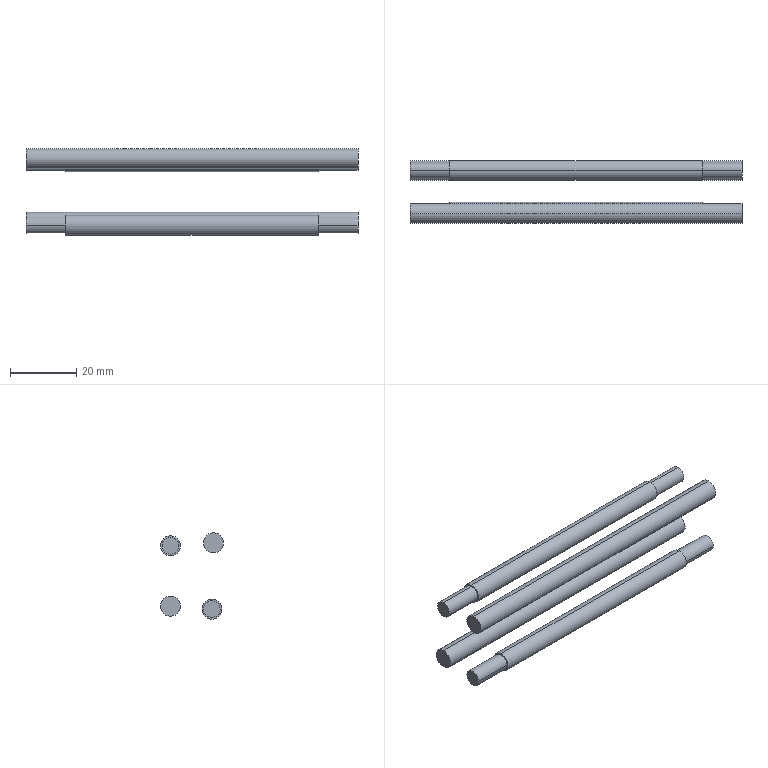Part | SolidWorks | features BaseBody 1, ICE 1 | 4 solids | 28 faces | box 100 x 19 x 26 mm | volume 10895 mm3 | cylinder 16 | plane 12 | commonest cylinder face diameters 5 x8 6 x8
STEP:
#1=CARTESIAN_POINT('',(-38.,-5.,-7.));
#2=VERTEX_POINT('',#1);
#3=CARTESIAN_POINT('',(-38.,-5.,-13.));
#4=VERTEX_POINT('',#3);
#5=CARTESIAN_POINT('',(-38.,-5.,-10.));
#6=DIRECTION('',(1.,0.,0.));
#7=DIRECTION('',(0.,0.,-1.));
#8=AXIS2_PLACEMENT_3D('',#5,#6,#7);
#9=CIRCLE('',#8,3.);
#10=EDGE_CURVE('',#2,#4,#9,.T.);
#11=ORIENTED_EDGE('',*,*,#10,.T.);
#12=CARTESIAN_POINT('',(38.,-5.,-13.));
#13=VERTEX_POINT('',#12);
#14=CARTESIAN_POINT('',(38.,-5.,-13.));
#15=DIRECTION('',(1.,0.,0.));
#16=VECTOR('',#15,1000.);
#17=LINE('',#14,#16);
#18=EDGE_CURVE('',#4,#13,#17,.T.);
#19=ORIENTED_EDGE('',*,*,#18,.T.);
#20=CARTESIAN_POINT('',(38.,-5.,-7.));
#21=VERTEX_POINT('',#20);
#22=CARTESIAN_POINT('',(38.,-5.,-10.));
#23=DIRECTION('',(-1.,0.,0.));
#24=DIRECTION('',(0.,0.,-1.));
#25=AXIS2_PLACEMENT_3D('',#22,#23,#24);
#26=CIRCLE('',#25,3.);
#27=EDGE_CURVE('',#13,#21,#26,.T.);
#28=ORIENTED_EDGE('',*,*,#27,.T.);
#29=CARTESIAN_POINT('',(38.,-5.,-7.));
#30=DIRECTION('',(1.,0.,0.));
#31=VECTOR('',#30,1000.);
#32=LINE('',#29,#31);
#33=EDGE_CURVE('',#2,#21,#32,.T.);
#34=ORIENTED_EDGE('',*,*,#33,.F.);
#35=EDGE_LOOP('',(#11,#19,#28,#34));
#36=FACE_OUTER_BOUND('',#35,.T.);
#37=CARTESIAN_POINT('',(38.,-5.,-10.));
#38=DIRECTION('',(1.,0.,0.));
#39=DIRECTION('',(0.,0.,1.));
#40=AXIS2_PLACEMENT_3D('',#37,#38,#39);
#41=CYLINDRICAL_SURFACE('',#40,3.);
#42=ADVANCED_FACE('',(#36),#41,.T.);
#43=CARTESIAN_POINT('',(-50.,-2.5,-10.));
#44=VERTEX_POINT('',#43);
#45=CARTESIAN_POINT('',(-50.,-7.5,-10.));
#46=VERTEX_POINT('',#45);
#47=CARTESIAN_POINT('',(-50.,-5.,-10.));
#48=DIRECTION('',(-1.,0.,0.));
#49=DIRECTION('',(0.,-1.,0.));
#50=AXIS2_PLACEMENT_3D('',#47,#48,#49);
#51=CIRCLE('',#50,2.5);
#52=EDGE_CURVE('',#44,#46,#51,.T.);
#53=ORIENTED_EDGE('',*,*,#52,.F.);
#54=CARTESIAN_POINT('',(-38.,-2.5,-10.));
#55=VERTEX_POINT('',#54);
#56=CARTESIAN_POINT('',(-50.,-2.5,-10.));
#57=DIRECTION('',(1.,0.,0.));
#58=VECTOR('',#57,1000.);
#59=LINE('',#56,#58);
#60=EDGE_CURVE('',#44,#55,#59,.T.);
#61=ORIENTED_EDGE('',*,*,#60,.T.);
#62=CARTESIAN_POINT('',(-38.,-7.5,-10.));
#63=VERTEX_POINT('',#62);
#64=CARTESIAN_POINT('',(-38.,-5.,-10.));
#65=DIRECTION('',(-1.,0.,0.));
#66=DIRECTION('',(0.,0.,-1.));
#67=AXIS2_PLACEMENT_3D('',#64,#65,#66);
#68=CIRCLE('',#67,2.5);
#69=EDGE_CURVE('',#55,#63,#68,.T.);
#70=ORIENTED_EDGE('',*,*,#69,.T.);
#71=CARTESIAN_POINT('',(-50.,-7.5,-10.));
#72=DIRECTION('',(1.,0.,0.));
#73=VECTOR('',#72,1000.);
#74=LINE('',#71,#73);
#75=EDGE_CURVE('',#46,#63,#74,.T.);
#76=ORIENTED_EDGE('',*,*,#75,.F.);
#77=EDGE_LOOP('',(#53,#61,#70,#76));
#78=FACE_OUTER_BOUND('',#77,.T.);
#79=CARTESIAN_POINT('',(-50.,-5.,-10.));
#80=DIRECTION('',(1.,0.,0.));
#81=DIRECTION('',(0.,-1.,0.));
#82=AXIS2_PLACEMENT_3D('',#79,#80,#81);
#83=CYLINDRICAL_SURFACE('',#82,2.5);
#84=ADVANCED_FACE('',(#78),#83,.T.);
#85=CARTESIAN_POINT('',(38.,-7.5,-10.));
#86=VERTEX_POINT('',#85);
#87=CARTESIAN_POINT('',(38.,-2.5,-10.));
#88=VERTEX_POINT('',#87);
#89=CARTESIAN_POINT('',(38.,-5.,-10.));
#90=DIRECTION('',(1.,0.,0.));
#91=DIRECTION('',(0.,0.,-1.));
#92=AXIS2_PLACEMENT_3D('',#89,#90,#91);
#93=CIRCLE('',#92,2.5);
#94=EDGE_CURVE('',#86,#88,#93,.T.);
#95=ORIENTED_EDGE('',*,*,#94,.T.);
#96=CARTESIAN_POINT('',(50.,-2.5,-10.));
#97=VERTEX_POINT('',#96);
#98=CARTESIAN_POINT('',(38.,-2.5,-10.));
#99=DIRECTION('',(1.,0.,0.));
#100=VECTOR('',#99,1000.);
#101=LINE('',#98,#100);
#102=EDGE_CURVE('',#88,#97,#101,.T.);
#103=ORIENTED_EDGE('',*,*,#102,.T.);
#104=CARTESIAN_POINT('',(50.,-7.5,-10.));
#105=VERTEX_POINT('',#104);
#106=CARTESIAN_POINT('',(50.,-5.,-10.));
#107=DIRECTION('',(-1.,0.,0.));
#108=DIRECTION('',(0.,-1.,0.));
#109=AXIS2_PLACEMENT_3D('',#106,#107,#108);
#110=CIRCLE('',#109,2.5);
#111=EDGE_CURVE('',#97,#105,#110,.T.);
#112=ORIENTED_EDGE('',*,*,#111,.T.);
#113=CARTESIAN_POINT('',(38.,-7.5,-10.));
#114=DIRECTION('',(1.,0.,0.));
#115=VECTOR('',#114,1000.);
#116=LINE('',#113,#115);
#117=EDGE_CURVE('',#86,#105,#116,.T.);
#118=ORIENTED_EDGE('',*,*,#117,.F.);
#119=EDGE_LOOP('',(#95,#103,#112,#118));
#120=FACE_OUTER_BOUND('',#119,.T.);
#121=CARTESIAN_POINT('',(38.,-5.,-10.));
#122=DIRECTION('',(1.,0.,0.));
#123=DIRECTION('',(0.,-1.,0.));
#124=AXIS2_PLACEMENT_3D('',#121,#122,#123);
#125=CYLINDRICAL_SURFACE('',#124,2.5);
#126=ADVANCED_FACE('',(#120),#125,.T.);
#127=CARTESIAN_POINT('',(50.,-5.,-10.));
#128=DIRECTION('',(-1.,0.,0.));
#129=DIRECTION('',(0.,-1.,0.));
#130=AXIS2_PLACEMENT_3D('',#127,#128,#129);
#131=CIRCLE('',#130,2.5);
#132=EDGE_CURVE('',#105,#97,#131,.T.);
#133=ORIENTED_EDGE('',*,*,#132,.F.);
#134=ORIENTED_EDGE('',*,*,#111,.F.);
#135=EDGE_LOOP('',(#133,#134));
#136=FACE_OUTER_BOUND('',#135,.T.);
#137=CARTESIAN_POINT('',(50.,-5.,-10.));
#138=DIRECTION('',(-1.,0.,0.));
#139=DIRECTION('',(0.,0.,1.));
#140=AXIS2_PLACEMENT_3D('',#137,#138,#139);
#141=PLANE('',#140);
#142=ADVANCED_FACE('',(#136),#141,.F.);
#143=ORIENTED_EDGE('',*,*,#102,.F.);
#144=CARTESIAN_POINT('',(38.,-5.,-10.));
#145=DIRECTION('',(1.,0.,0.));
#146=DIRECTION('',(0.,0.,-1.));
#147=AXIS2_PLACEMENT_3D('',#144,#145,#146);
#148=CIRCLE('',#147,2.5);
#149=EDGE_CURVE('',#88,#86,#148,.T.);
#150=ORIENTED_EDGE('',*,*,#149,.T.);
#151=ORIENTED_EDGE('',*,*,#117,.T.);
#152=ORIENTED_EDGE('',*,*,#132,.T.);
#153=EDGE_LOOP('',(#143,#150,#151,#152));
#154=FACE_OUTER_BOUND('',#153,.T.);
#155=CARTESIAN_POINT('',(38.,-5.,-10.));
#156=DIRECTION('',(1.,0.,0.));
#157=DIRECTION('',(0.,-1.,0.));
#158=AXIS2_PLACEMENT_3D('',#155,#156,#157);
#159=CYLINDRICAL_SURFACE('',#158,2.5);
#160=ADVANCED_FACE('',(#154),#159,.T.);
#161=CARTESIAN_POINT('',(38.,-5.,-10.));
#162=DIRECTION('',(-1.,0.,0.));
#163=DIRECTION('',(0.,0.,-1.));
#164=AXIS2_PLACEMENT_3D('',#161,#162,#163);
#165=CIRCLE('',#164,3.);
#166=EDGE_CURVE('',#21,#13,#165,.T.);
#167=ORIENTED_EDGE('',*,*,#166,.F.);
#168=ORIENTED_EDGE('',*,*,#27,.F.);
#169=EDGE_LOOP('',(#167,#168));
#170=FACE_OUTER_BOUND('',#169,.T.);
#171=ORIENTED_EDGE('',*,*,#94,.F.);
#172=ORIENTED_EDGE('',*,*,#149,.F.);
#173=EDGE_LOOP('',(#171,#172));
#174=FACE_BOUND('',#173,.T.);
#175=CARTESIAN_POINT('',(38.,0.,0.));
#176=DIRECTION('',(1.,0.,0.));
#177=DIRECTION('',(0.,0.,-1.));
#178=AXIS2_PLACEMENT_3D('',#175,#176,#177);
#179=PLANE('',#178);
#180=ADVANCED_FACE('',(#170,#174),#179,.T.);
#181=CARTESIAN_POINT('',(-50.,-5.,-10.));
#182=DIRECTION('',(-1.,0.,0.));
#183=DIRECTION('',(0.,-1.,0.));
#184=AXIS2_PLACEMENT_3D('',#181,#182,#183);
#185=CIRCLE('',#184,2.5);
#186=EDGE_CURVE('',#46,#44,#185,.T.);
#187=ORIENTED_EDGE('',*,*,#186,.T.);
#188=ORIENTED_EDGE('',*,*,#52,.T.);
#189=EDGE_LOOP('',(#187,#188));
#190=FACE_OUTER_BOUND('',#189,.T.);
#191=CARTESIAN_POINT('',(-50.,-7.5,-10.));
#192=DIRECTION('',(1.,0.,0.));
#193=DIRECTION('',(0.,1.,0.));
#194=AXIS2_PLACEMENT_3D('',#191,#192,#193);
#195=PLANE('',#194);
#196=ADVANCED_FACE('',(#190),#195,.F.);
#197=ORIENTED_EDGE('',*,*,#60,.F.);
#198=ORIENTED_EDGE('',*,*,#186,.F.);
#199=ORIENTED_EDGE('',*,*,#75,.T.);
#200=CARTESIAN_POINT('',(-38.,-5.,-10.));
#201=DIRECTION('',(-1.,0.,0.));
#202=DIRECTION('',(0.,0.,-1.));
#203=AXIS2_PLACEMENT_3D('',#200,#201,#202);
#204=CIRCLE('',#203,2.5);
#205=EDGE_CURVE('',#63,#55,#204,.T.);
#206=ORIENTED_EDGE('',*,*,#205,.T.);
#207=EDGE_LOOP('',(#197,#198,#199,#206));
#208=FACE_OUTER_BOUND('',#207,.T.);
#209=CARTESIAN_POINT('',(-50.,-5.,-10.));
#210=DIRECTION('',(1.,0.,0.));
#211=DIRECTION('',(0.,-1.,0.));
#212=AXIS2_PLACEMENT_3D('',#209,#210,#211);
#213=CYLINDRICAL_SURFACE('',#212,2.5);
#214=ADVANCED_FACE('',(#208),#213,.T.);
#215=ORIENTED_EDGE('',*,*,#10,.F.);
#216=CARTESIAN_POINT('',(-38.,-5.,-10.));
#217=DIRECTION('',(1.,0.,0.));
#218=DIRECTION('',(0.,0.,-1.));
#219=AXIS2_PLACEMENT_3D('',#216,#217,#218);
#220=CIRCLE('',#219,3.);
#221=EDGE_CURVE('',#4,#2,#220,.T.);
#222=ORIENTED_EDGE('',*,*,#221,.F.);
#223=EDGE_LOOP('',(#215,#222));
#224=FACE_OUTER_BOUND('',#223,.T.);
#225=ORIENTED_EDGE('',*,*,#205,.F.);
#226=ORIENTED_EDGE('',*,*,#69,.F.);
#227=EDGE_LOOP('',(#225,#226));
#228=FACE_BOUND('',#227,.T.);
#229=CARTESIAN_POINT('',(-38.,-5.,-10.));
#230=DIRECTION('',(1.,0.,0.));
#231=DIRECTION('',(0.,1.,0.));
#232=AXIS2_PLACEMENT_3D('',#229,#230,#231);
#233=PLANE('',#232);
#234=ADVANCED_FACE('',(#224,#228),#233,.F.);
#235=ORIENTED_EDGE('',*,*,#18,.F.);
#236=ORIENTED_EDGE('',*,*,#221,.T.);
#237=ORIENTED_EDGE('',*,*,#33,.T.);
#238=ORIENTED_EDGE('',*,*,#166,.T.);
#239=EDGE_LOOP('',(#235,#236,#237,#238));
#240=FACE_OUTER_BOUND('',#239,.T.);
#241=CARTESIAN_POINT('',(38.,-5.,-10.));
#242=DIRECTION('',(1.,0.,0.));
#243=DIRECTION('',(0.,0.,1.));
#244=AXIS2_PLACEMENT_3D('',#241,#242,#243);
#245=CYLINDRICAL_SURFACE('',#244,3.);
#246=ADVANCED_FACE('',(#240),#245,.T.);
#247=CLOSED_SHELL('',(#42,#84,#126,#142,#160,#180,#196,#214,#234,#246));
#248=MANIFOLD_SOLID_BREP('',#247);
#249=CARTESIAN_POINT('',(-50.,-5.5,13.));
#250=VERTEX_POINT('',#249);
#251=CARTESIAN_POINT('',(-50.,-5.5,7.));
#252=VERTEX_POINT('',#251);
#253=CARTESIAN_POINT('',(-50.,-5.5,10.));
#254=DIRECTION('',(1.,0.,0.));
#255=DIRECTION('',(0.,0.,-1.));
#256=AXIS2_PLACEMENT_3D('',#253,#254,#255);
#257=CIRCLE('',#256,3.);
#258=EDGE_CURVE('',#250,#252,#257,.T.);
#259=ORIENTED_EDGE('',*,*,#258,.T.);
#260=CARTESIAN_POINT('',(50.,-5.5,7.));
#261=VERTEX_POINT('',#260);
#262=CARTESIAN_POINT('',(50.,-5.5,7.));
#263=DIRECTION('',(1.,0.,0.));
#264=VECTOR('',#263,1000.);
#265=LINE('',#262,#264);
#266=EDGE_CURVE('',#252,#261,#265,.T.);
#267=ORIENTED_EDGE('',*,*,#266,.T.);
#268=CARTESIAN_POINT('',(50.,-5.5,13.));
#269=VERTEX_POINT('',#268);
#270=CARTESIAN_POINT('',(50.,-5.5,10.));
#271=DIRECTION('',(1.,0.,0.));
#272=DIRECTION('',(0.,0.,-1.));
#273=AXIS2_PLACEMENT_3D('',#270,#271,#272);
#274=CIRCLE('',#273,3.);
#275=EDGE_CURVE('',#269,#261,#274,.T.);
#276=ORIENTED_EDGE('',*,*,#275,.F.);
#277=CARTESIAN_POINT('',(50.,-5.5,13.));
#278=DIRECTION('',(1.,0.,0.));
#279=VECTOR('',#278,1000.);
#280=LINE('',#277,#279);
#281=EDGE_CURVE('',#250,#269,#280,.T.);
#282=ORIENTED_EDGE('',*,*,#281,.F.);
#283=EDGE_LOOP('',(#259,#267,#276,#282));
#284=FACE_OUTER_BOUND('',#283,.T.);
#285=CARTESIAN_POINT('',(50.,-5.5,10.));
#286=DIRECTION('',(1.,0.,0.));
#287=DIRECTION('',(0.,0.,1.));
#288=AXIS2_PLACEMENT_3D('',#285,#286,#287);
#289=CYLINDRICAL_SURFACE('',#288,3.);
#290=ADVANCED_FACE('',(#284),#289,.T.);
#291=ORIENTED_EDGE('',*,*,#258,.F.);
#292=CARTESIAN_POINT('',(-50.,-5.5,10.));
#293=DIRECTION('',(1.,0.,0.));
#294=DIRECTION('',(0.,0.,-1.));
#295=AXIS2_PLACEMENT_3D('',#292,#293,#294);
#296=CIRCLE('',#295,3.);
#297=EDGE_CURVE('',#252,#250,#296,.T.);
#298=ORIENTED_EDGE('',*,*,#297,.F.);
#299=EDGE_LOOP('',(#291,#298));
#300=FACE_OUTER_BOUND('',#299,.T.);
#301=CARTESIAN_POINT('',(-50.,-5.5,10.));
#302=DIRECTION('',(1.,0.,0.));
#303=DIRECTION('',(0.,1.,0.));
#304=AXIS2_PLACEMENT_3D('',#301,#302,#303);
#305=PLANE('',#304);
#306=ADVANCED_FACE('',(#300),#305,.F.);
#307=ORIENTED_EDGE('',*,*,#266,.F.);
#308=ORIENTED_EDGE('',*,*,#297,.T.);
#309=ORIENTED_EDGE('',*,*,#281,.T.);
#310=CARTESIAN_POINT('',(50.,-5.5,10.));
#311=DIRECTION('',(1.,0.,0.));
#312=DIRECTION('',(0.,0.,-1.));
#313=AXIS2_PLACEMENT_3D('',#310,#311,#312);
#314=CIRCLE('',#313,3.);
#315=EDGE_CURVE('',#261,#269,#314,.T.);
#316=ORIENTED_EDGE('',*,*,#315,.F.);
#317=EDGE_LOOP('',(#307,#308,#309,#316));
#318=FACE_OUTER_BOUND('',#317,.T.);
#319=CARTESIAN_POINT('',(50.,-5.5,10.));
#320=DIRECTION('',(1.,0.,0.));
#321=DIRECTION('',(0.,0.,1.));
#322=AXIS2_PLACEMENT_3D('',#319,#320,#321);
#323=CYLINDRICAL_SURFACE('',#322,3.);
#324=ADVANCED_FACE('',(#318),#323,.T.);
#325=ORIENTED_EDGE('',*,*,#275,.T.);
#326=ORIENTED_EDGE('',*,*,#315,.T.);
#327=EDGE_LOOP('',(#325,#326));
#328=FACE_OUTER_BOUND('',#327,.T.);
#329=CARTESIAN_POINT('',(50.,-5.5,10.));
#330=DIRECTION('',(1.,0.,0.));
#331=DIRECTION('',(0.,1.,0.));
#332=AXIS2_PLACEMENT_3D('',#329,#330,#331);
#333=PLANE('',#332);
#334=ADVANCED_FACE('',(#328),#333,.T.);
#335=CLOSED_SHELL('',(#290,#306,#324,#334));
#336=MANIFOLD_SOLID_BREP('',#335);
#337=CARTESIAN_POINT('',(38.,7.5,6.6));
#338=VERTEX_POINT('',#337);
#339=CARTESIAN_POINT('',(38.,7.5,11.6));
#340=VERTEX_POINT('',#339);
#341=CARTESIAN_POINT('',(38.,7.5,9.1));
#342=DIRECTION('',(1.,0.,0.));
#343=DIRECTION('',(0.,0.,-1.));
#344=AXIS2_PLACEMENT_3D('',#341,#342,#343);
#345=CIRCLE('',#344,2.5);
#346=EDGE_CURVE('',#338,#340,#345,.T.);
#347=ORIENTED_EDGE('',*,*,#346,.T.);
#348=CARTESIAN_POINT('',(50.,7.5,11.6));
#349=VERTEX_POINT('',#348);
#350=CARTESIAN_POINT('',(38.,7.5,11.6));
#351=DIRECTION('',(1.,0.,0.));
#352=VECTOR('',#351,1000.);
#353=LINE('',#350,#352);
#354=EDGE_CURVE('',#340,#349,#353,.T.);
#355=ORIENTED_EDGE('',*,*,#354,.T.);
#356=CARTESIAN_POINT('',(50.,7.5,6.6));
#357=VERTEX_POINT('',#356);
#358=CARTESIAN_POINT('',(50.,7.5,9.1));
#359=DIRECTION('',(-1.,0.,0.));
#360=DIRECTION('',(0.,0.,1.));
#361=AXIS2_PLACEMENT_3D('',#358,#359,#360);
#362=CIRCLE('',#361,2.5);
#363=EDGE_CURVE('',#349,#357,#362,.T.);
#364=ORIENTED_EDGE('',*,*,#363,.T.);
#365=CARTESIAN_POINT('',(38.,7.5,6.6));
#366=DIRECTION('',(1.,0.,0.));
#367=VECTOR('',#366,1000.);
#368=LINE('',#365,#367);
#369=EDGE_CURVE('',#338,#357,#368,.T.);
#370=ORIENTED_EDGE('',*,*,#369,.F.);
#371=EDGE_LOOP('',(#347,#355,#364,#370));
#372=FACE_OUTER_BOUND('',#371,.T.);
#373=CARTESIAN_POINT('',(38.,7.5,9.1));
#374=DIRECTION('',(1.,0.,0.));
#375=DIRECTION('',(0.,0.,-1.));
#376=AXIS2_PLACEMENT_3D('',#373,#374,#375);
#377=CYLINDRICAL_SURFACE('',#376,2.5);
#378=ADVANCED_FACE('',(#372),#377,.T.);
#379=CARTESIAN_POINT('',(-50.,7.5,6.6));
#380=VERTEX_POINT('',#379);
#381=CARTESIAN_POINT('',(-50.,7.5,11.6));
#382=VERTEX_POINT('',#381);
#383=CARTESIAN_POINT('',(-50.,7.5,9.1));
#384=DIRECTION('',(-1.,0.,0.));
#385=DIRECTION('',(0.,0.,1.));
#386=AXIS2_PLACEMENT_3D('',#383,#384,#385);
#387=CIRCLE('',#386,2.5);
#388=EDGE_CURVE('',#380,#382,#387,.T.);
#389=ORIENTED_EDGE('',*,*,#388,.F.);
#390=CARTESIAN_POINT('',(-38.,7.5,6.6));
#391=VERTEX_POINT('',#390);
#392=CARTESIAN_POINT('',(-50.,7.5,6.6));
#393=DIRECTION('',(1.,0.,0.));
#394=VECTOR('',#393,1000.);
#395=LINE('',#392,#394);
#396=EDGE_CURVE('',#380,#391,#395,.T.);
#397=ORIENTED_EDGE('',*,*,#396,.T.);
#398=CARTESIAN_POINT('',(-38.,7.5,11.6));
#399=VERTEX_POINT('',#398);
#400=CARTESIAN_POINT('',(-38.,7.5,9.1));
#401=DIRECTION('',(-1.,0.,0.));
#402=DIRECTION('',(0.,0.,-1.));
#403=AXIS2_PLACEMENT_3D('',#400,#401,#402);
#404=CIRCLE('',#403,2.5);
#405=EDGE_CURVE('',#391,#399,#404,.T.);
#406=ORIENTED_EDGE('',*,*,#405,.T.);
#407=CARTESIAN_POINT('',(-50.,7.5,11.6));
#408=DIRECTION('',(1.,0.,0.));
#409=VECTOR('',#408,1000.);
#410=LINE('',#407,#409);
#411=EDGE_CURVE('',#382,#399,#410,.T.);
#412=ORIENTED_EDGE('',*,*,#411,.F.);
#413=EDGE_LOOP('',(#389,#397,#406,#412));
#414=FACE_OUTER_BOUND('',#413,.T.);
#415=CARTESIAN_POINT('',(-50.,7.5,9.1));
#416=DIRECTION('',(1.,0.,0.));
#417=DIRECTION('',(0.,0.,1.));
#418=AXIS2_PLACEMENT_3D('',#415,#416,#417);
#419=CYLINDRICAL_SURFACE('',#418,2.5);
#420=ADVANCED_FACE('',(#414),#419,.T.);
#421=CARTESIAN_POINT('',(-38.,7.5,12.1));
#422=VERTEX_POINT('',#421);
#423=CARTESIAN_POINT('',(-38.,7.5,6.1));
#424=VERTEX_POINT('',#423);
#425=CARTESIAN_POINT('',(-38.,7.5,9.1));
#426=DIRECTION('',(1.,0.,0.));
#427=DIRECTION('',(0.,0.,-1.));
#428=AXIS2_PLACEMENT_3D('',#425,#426,#427);
#429=CIRCLE('',#428,3.);
#430=EDGE_CURVE('',#422,#424,#429,.T.);
#431=ORIENTED_EDGE('',*,*,#430,.T.);
#432=CARTESIAN_POINT('',(38.,7.5,6.1));
#433=VERTEX_POINT('',#432);
#434=CARTESIAN_POINT('',(38.,7.5,6.1));
#435=DIRECTION('',(1.,0.,0.));
#436=VECTOR('',#435,1000.);
#437=LINE('',#434,#436);
#438=EDGE_CURVE('',#424,#433,#437,.T.);
#439=ORIENTED_EDGE('',*,*,#438,.T.);
#440=CARTESIAN_POINT('',(38.,7.5,12.1));
#441=VERTEX_POINT('',#440);
#442=CARTESIAN_POINT('',(38.,7.5,9.1));
#443=DIRECTION('',(-1.,0.,0.));
#444=DIRECTION('',(0.,0.,-1.));
#445=AXIS2_PLACEMENT_3D('',#442,#443,#444);
#446=CIRCLE('',#445,3.);
#447=EDGE_CURVE('',#433,#441,#446,.T.);
#448=ORIENTED_EDGE('',*,*,#447,.T.);
#449=CARTESIAN_POINT('',(38.,7.5,12.1));
#450=DIRECTION('',(1.,0.,0.));
#451=VECTOR('',#450,1000.);
#452=LINE('',#449,#451);
#453=EDGE_CURVE('',#422,#441,#452,.T.);
#454=ORIENTED_EDGE('',*,*,#453,.F.);
#455=EDGE_LOOP('',(#431,#439,#448,#454));
#456=FACE_OUTER_BOUND('',#455,.T.);
#457=CARTESIAN_POINT('',(38.,7.5,9.1));
#458=DIRECTION('',(1.,0.,0.));
#459=DIRECTION('',(0.,0.,1.));
#460=AXIS2_PLACEMENT_3D('',#457,#458,#459);
#461=CYLINDRICAL_SURFACE('',#460,3.);
#462=ADVANCED_FACE('',(#456),#461,.T.);
#463=ORIENTED_EDGE('',*,*,#430,.F.);
#464=CARTESIAN_POINT('',(-38.,7.5,9.1));
#465=DIRECTION('',(1.,0.,0.));
#466=DIRECTION('',(0.,0.,-1.));
#467=AXIS2_PLACEMENT_3D('',#464,#465,#466);
#468=CIRCLE('',#467,3.);
#469=EDGE_CURVE('',#424,#422,#468,.T.);
#470=ORIENTED_EDGE('',*,*,#469,.F.);
#471=EDGE_LOOP('',(#463,#470));
#472=FACE_OUTER_BOUND('',#471,.T.);
#473=CARTESIAN_POINT('',(-38.,7.5,9.1));
#474=DIRECTION('',(-1.,0.,0.));
#475=DIRECTION('',(0.,0.,-1.));
#476=AXIS2_PLACEMENT_3D('',#473,#474,#475);
#477=CIRCLE('',#476,2.5);
#478=EDGE_CURVE('',#399,#391,#477,.T.);
#479=ORIENTED_EDGE('',*,*,#478,.F.);
#480=ORIENTED_EDGE('',*,*,#405,.F.);
#481=EDGE_LOOP('',(#479,#480));
#482=FACE_BOUND('',#481,.T.);
#483=CARTESIAN_POINT('',(-38.,7.5,9.1));
#484=DIRECTION('',(1.,0.,0.));
#485=DIRECTION('',(0.,1.,0.));
#486=AXIS2_PLACEMENT_3D('',#483,#484,#485);
#487=PLANE('',#486);
#488=ADVANCED_FACE('',(#472,#482),#487,.F.);
#489=ORIENTED_EDGE('',*,*,#438,.F.);
#490=ORIENTED_EDGE('',*,*,#469,.T.);
#491=ORIENTED_EDGE('',*,*,#453,.T.);
#492=CARTESIAN_POINT('',(38.,7.5,9.1));
#493=DIRECTION('',(-1.,0.,0.));
#494=DIRECTION('',(0.,0.,-1.));
#495=AXIS2_PLACEMENT_3D('',#492,#493,#494);
#496=CIRCLE('',#495,3.);
#497=EDGE_CURVE('',#441,#433,#496,.T.);
#498=ORIENTED_EDGE('',*,*,#497,.T.);
#499=EDGE_LOOP('',(#489,#490,#491,#498));
#500=FACE_OUTER_BOUND('',#499,.T.);
#501=CARTESIAN_POINT('',(38.,7.5,9.1));
#502=DIRECTION('',(1.,0.,0.));
#503=DIRECTION('',(0.,0.,1.));
#504=AXIS2_PLACEMENT_3D('',#501,#502,#503);
#505=CYLINDRICAL_SURFACE('',#504,3.);
#506=ADVANCED_FACE('',(#500),#505,.T.);
#507=ORIENTED_EDGE('',*,*,#396,.F.);
#508=CARTESIAN_POINT('',(-50.,7.5,9.1));
#509=DIRECTION('',(-1.,0.,0.));
#510=DIRECTION('',(0.,0.,1.));
#511=AXIS2_PLACEMENT_3D('',#508,#509,#510);
#512=CIRCLE('',#511,2.5);
#513=EDGE_CURVE('',#382,#380,#512,.T.);
#514=ORIENTED_EDGE('',*,*,#513,.F.);
#515=ORIENTED_EDGE('',*,*,#411,.T.);
#516=ORIENTED_EDGE('',*,*,#478,.T.);
#517=EDGE_LOOP('',(#507,#514,#515,#516));
#518=FACE_OUTER_BOUND('',#517,.T.);
#519=CARTESIAN_POINT('',(-50.,7.5,9.1));
#520=DIRECTION('',(1.,0.,0.));
#521=DIRECTION('',(0.,0.,1.));
#522=AXIS2_PLACEMENT_3D('',#519,#520,#521);
#523=CYLINDRICAL_SURFACE('',#522,2.5);
#524=ADVANCED_FACE('',(#518),#523,.T.);
#525=ORIENTED_EDGE('',*,*,#513,.T.);
#526=ORIENTED_EDGE('',*,*,#388,.T.);
#527=EDGE_LOOP('',(#525,#526));
#528=FACE_OUTER_BOUND('',#527,.T.);
#529=CARTESIAN_POINT('',(-50.,7.5,11.6));
#530=DIRECTION('',(1.,0.,0.));
#531=DIRECTION('',(0.,0.,-1.));
#532=AXIS2_PLACEMENT_3D('',#529,#530,#531);
#533=PLANE('',#532);
#534=ADVANCED_FACE('',(#528),#533,.F.);
#535=ORIENTED_EDGE('',*,*,#354,.F.);
#536=CARTESIAN_POINT('',(38.,7.5,9.1));
#537=DIRECTION('',(1.,0.,0.));
#538=DIRECTION('',(0.,0.,-1.));
#539=AXIS2_PLACEMENT_3D('',#536,#537,#538);
#540=CIRCLE('',#539,2.5);
#541=EDGE_CURVE('',#340,#338,#540,.T.);
#542=ORIENTED_EDGE('',*,*,#541,.T.);
#543=ORIENTED_EDGE('',*,*,#369,.T.);
#544=CARTESIAN_POINT('',(50.,7.5,9.1));
#545=DIRECTION('',(-1.,0.,0.));
#546=DIRECTION('',(0.,0.,1.));
#547=AXIS2_PLACEMENT_3D('',#544,#545,#546);
#548=CIRCLE('',#547,2.5);
#549=EDGE_CURVE('',#357,#349,#548,.T.);
#550=ORIENTED_EDGE('',*,*,#549,.T.);
#551=EDGE_LOOP('',(#535,#542,#543,#550));
#552=FACE_OUTER_BOUND('',#551,.T.);
#553=CARTESIAN_POINT('',(38.,7.5,9.1));
#554=DIRECTION('',(1.,0.,0.));
#555=DIRECTION('',(0.,0.,-1.));
#556=AXIS2_PLACEMENT_3D('',#553,#554,#555);
#557=CYLINDRICAL_SURFACE('',#556,2.5);
#558=ADVANCED_FACE('',(#552),#557,.T.);
#559=ORIENTED_EDGE('',*,*,#497,.F.);
#560=ORIENTED_EDGE('',*,*,#447,.F.);
#561=EDGE_LOOP('',(#559,#560));
#562=FACE_OUTER_BOUND('',#561,.T.);
#563=ORIENTED_EDGE('',*,*,#346,.F.);
#564=ORIENTED_EDGE('',*,*,#541,.F.);
#565=EDGE_LOOP('',(#563,#564));
#566=FACE_BOUND('',#565,.T.);
#567=CARTESIAN_POINT('',(38.,0.,0.));
#568=DIRECTION('',(1.,0.,0.));
#569=DIRECTION('',(0.,0.,-1.));
#570=AXIS2_PLACEMENT_3D('',#567,#568,#569);
#571=PLANE('',#570);
#572=ADVANCED_FACE('',(#562,#566),#571,.T.);
#573=ORIENTED_EDGE('',*,*,#549,.F.);
#574=ORIENTED_EDGE('',*,*,#363,.F.);
#575=EDGE_LOOP('',(#573,#574));
#576=FACE_OUTER_BOUND('',#575,.T.);
#577=CARTESIAN_POINT('',(50.,7.5,9.1));
#578=DIRECTION('',(-1.,0.,0.));
#579=DIRECTION('',(0.,0.,1.));
#580=AXIS2_PLACEMENT_3D('',#577,#578,#579);
#581=PLANE('',#580);
#582=ADVANCED_FACE('',(#576),#581,.F.);
#583=CLOSED_SHELL('',(#378,#420,#462,#488,#506,#524,#534,#558,#572,#582));
#584=MANIFOLD_SOLID_BREP('',#583);
#585=CARTESIAN_POINT('',(-50.,7.5,-6.1));
#586=VERTEX_POINT('',#585);
#587=CARTESIAN_POINT('',(-50.,7.5,-12.1));
#588=VERTEX_POINT('',#587);
#589=CARTESIAN_POINT('',(-50.,7.5,-9.1));
#590=DIRECTION('',(1.,0.,0.));
#591=DIRECTION('',(0.,0.,-1.));
#592=AXIS2_PLACEMENT_3D('',#589,#590,#591);
#593=CIRCLE('',#592,3.);
#594=EDGE_CURVE('',#586,#588,#593,.T.);
#595=ORIENTED_EDGE('',*,*,#594,.T.);
#596=CARTESIAN_POINT('',(50.,7.5,-12.1));
#597=VERTEX_POINT('',#596);
#598=CARTESIAN_POINT('',(50.,7.5,-12.1));
#599=DIRECTION('',(1.,0.,0.));
#600=VECTOR('',#599,1000.);
#601=LINE('',#598,#600);
#602=EDGE_CURVE('',#588,#597,#601,.T.);
#603=ORIENTED_EDGE('',*,*,#602,.T.);
#604=CARTESIAN_POINT('',(50.,7.5,-6.1));
#605=VERTEX_POINT('',#604);
#606=CARTESIAN_POINT('',(50.,7.5,-9.1));
#607=DIRECTION('',(1.,0.,0.));
#608=DIRECTION('',(0.,0.,-1.));
#609=AXIS2_PLACEMENT_3D('',#606,#607,#608);
#610=CIRCLE('',#609,3.);
#611=EDGE_CURVE('',#605,#597,#610,.T.);
#612=ORIENTED_EDGE('',*,*,#611,.F.);
#613=CARTESIAN_POINT('',(50.,7.5,-6.1));
#614=DIRECTION('',(1.,0.,0.));
#615=VECTOR('',#614,1000.);
#616=LINE('',#613,#615);
#617=EDGE_CURVE('',#586,#605,#616,.T.);
#618=ORIENTED_EDGE('',*,*,#617,.F.);
#619=EDGE_LOOP('',(#595,#603,#612,#618));
#620=FACE_OUTER_BOUND('',#619,.T.);
#621=CARTESIAN_POINT('',(50.,7.5,-9.1));
#622=DIRECTION('',(1.,0.,0.));
#623=DIRECTION('',(0.,0.,1.));
#624=AXIS2_PLACEMENT_3D('',#621,#622,#623);
#625=CYLINDRICAL_SURFACE('',#624,3.);
#626=ADVANCED_FACE('',(#620),#625,.T.);
#627=ORIENTED_EDGE('',*,*,#611,.T.);
#628=CARTESIAN_POINT('',(50.,7.5,-9.1));
#629=DIRECTION('',(1.,0.,0.));
#630=DIRECTION('',(0.,0.,-1.));
#631=AXIS2_PLACEMENT_3D('',#628,#629,#630);
#632=CIRCLE('',#631,3.);
#633=EDGE_CURVE('',#597,#605,#632,.T.);
#634=ORIENTED_EDGE('',*,*,#633,.T.);
#635=EDGE_LOOP('',(#627,#634));
#636=FACE_OUTER_BOUND('',#635,.T.);
#637=CARTESIAN_POINT('',(50.,7.5,-9.1));
#638=DIRECTION('',(1.,0.,0.));
#639=DIRECTION('',(0.,1.,0.));
#640=AXIS2_PLACEMENT_3D('',#637,#638,#639);
#641=PLANE('',#640);
#642=ADVANCED_FACE('',(#636),#641,.T.);
#643=ORIENTED_EDGE('',*,*,#594,.F.);
#644=CARTESIAN_POINT('',(-50.,7.5,-9.1));
#645=DIRECTION('',(1.,0.,0.));
#646=DIRECTION('',(0.,0.,-1.));
#647=AXIS2_PLACEMENT_3D('',#644,#645,#646);
#648=CIRCLE('',#647,3.);
#649=EDGE_CURVE('',#588,#586,#648,.T.);
#650=ORIENTED_EDGE('',*,*,#649,.F.);
#651=EDGE_LOOP('',(#643,#650));
#652=FACE_OUTER_BOUND('',#651,.T.);
#653=CARTESIAN_POINT('',(-50.,7.5,-9.1));
#654=DIRECTION('',(1.,0.,0.));
#655=DIRECTION('',(0.,1.,0.));
#656=AXIS2_PLACEMENT_3D('',#653,#654,#655);
#657=PLANE('',#656);
#658=ADVANCED_FACE('',(#652),#657,.F.);
#659=ORIENTED_EDGE('',*,*,#602,.F.);
#660=ORIENTED_EDGE('',*,*,#649,.T.);
#661=ORIENTED_EDGE('',*,*,#617,.T.);
#662=ORIENTED_EDGE('',*,*,#633,.F.);
#663=EDGE_LOOP('',(#659,#660,#661,#662));
#664=FACE_OUTER_BOUND('',#663,.T.);
#665=CARTESIAN_POINT('',(50.,7.5,-9.1));
#666=DIRECTION('',(1.,0.,0.));
#667=DIRECTION('',(0.,0.,1.));
#668=AXIS2_PLACEMENT_3D('',#665,#666,#667);
#669=CYLINDRICAL_SURFACE('',#668,3.);
#670=ADVANCED_FACE('',(#664),#669,.T.);
#671=CLOSED_SHELL('',(#626,#642,#658,#670));
#672=MANIFOLD_SOLID_BREP('',#671);
#673=CARTESIAN_POINT('',(0.,0.,0.));
#674=DIRECTION('',(0.,0.,1.));
#675=DIRECTION('',(1.,0.,0.));
#676=AXIS2_PLACEMENT_3D('',#673,#674,#675);
#677=(LENGTH_UNIT()NAMED_UNIT(*)SI_UNIT(.MILLI.,.METRE.));
#678=UNCERTAINTY_MEASURE_WITH_UNIT(LENGTH_MEASURE(0.00001),#677,'','');
#679=(NAMED_UNIT(*)PLANE_ANGLE_UNIT()SI_UNIT($,.RADIAN.));
#680=(NAMED_UNIT(*)SI_UNIT($,.STERADIAN.)SOLID_ANGLE_UNIT());
#681=(GEOMETRIC_REPRESENTATION_CONTEXT(3)GLOBAL_UNCERTAINTY_ASSIGNED_CONTEXT((#678))GLOBAL_UNIT_ASSIGNED_CONTEXT((#677,#679,#680))REPRESENTATION_CONTEXT('',''));
#682=ADVANCED_BREP_SHAPE_REPRESENTATION('',(#248,#336,#584,#672,#676),#681);